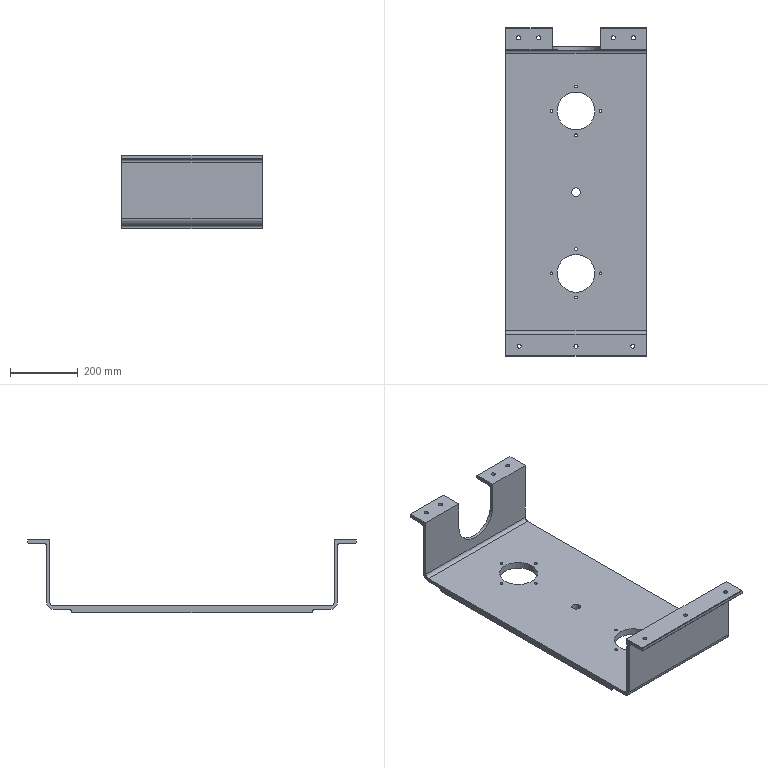Part | NX | features BREP 1 | 1 solid | 75 faces | box 416 x 972 x 217 mm | volume 7985494 mm3 | cylinder 46 | plane 29 | commonest cylinder face diameters 8 x16 12 x14 16 x5 112 x4 20 x2 25 x2